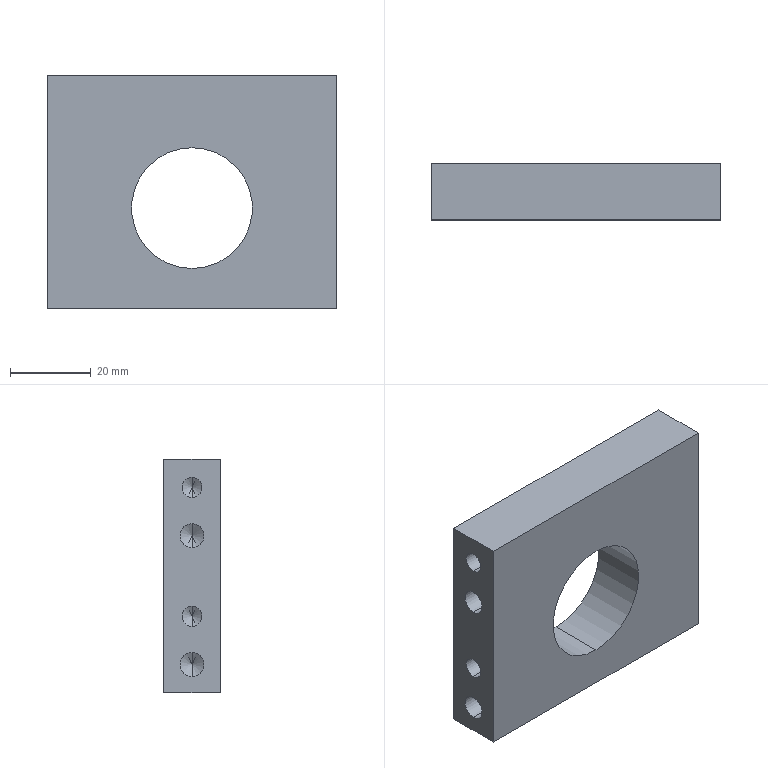Part | STEP file | OP10-141_inclined plate (F) | 1 solid | 56 faces | box 72 x 14 x 58 mm | volume 45441 mm3 | cylinder 26 | cone 24 | plane 6 | commonest cylinder face diameters 4.2 x8 5 x8 6 x8 30 x2